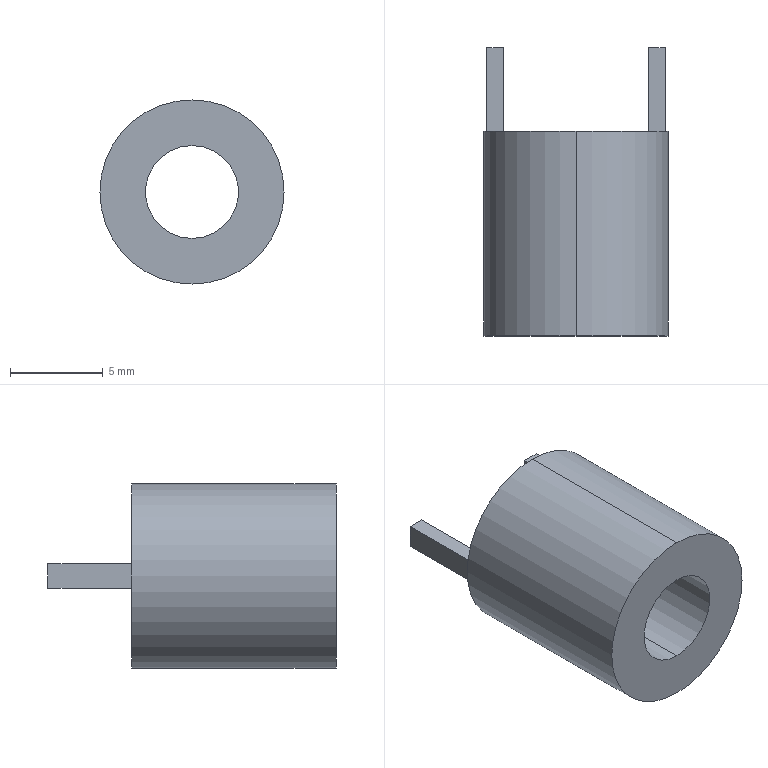Part | STEP file | 1 solid | 16 faces | box 9.9 x 15.5 x 9.9 mm | volume 641.291 mm3 | plane 12 | cylinder 4 | commonest cylinder face diameters 5 x2 9.9 x2
STEP:
#1=CARTESIAN_POINT('',(0.,0.,0.));
#2=DIRECTION('',(0.,0.,1.));
#3=DIRECTION('',(1.,0.,0.));
#4=AXIS2_PLACEMENT_3D('',#1,#2,#3);
#5=CARTESIAN_POINT('',(0.,0.,2.5));
#6=VERTEX_POINT('',#5);
#7=CARTESIAN_POINT('',(0.,11.,2.5));
#8=VERTEX_POINT('',#7);
#9=CARTESIAN_POINT('',(0.,11.,2.5));
#10=DIRECTION('',(0.,1.,0.));
#11=VECTOR('',#10,1.);
#12=LINE('',#9,#11);
#13=CARTESIAN_POINT('',(0.,11.,0.));
#14=DIRECTION('',(0.,1.,0.));
#15=DIRECTION('',(0.,0.,1.));
#16=AXIS2_PLACEMENT_3D('',#13,#14,#15);
#17=CYLINDRICAL_SURFACE('',#16,2.5);
#18=CARTESIAN_POINT('',(6.283,0.));
#19=DIRECTION('',(0.,1.));
#20=VECTOR('',#19,1.);
#21=LINE('',#18,#20);
#22=(GEOMETRIC_REPRESENTATION_CONTEXT(2)PARAMETRIC_REPRESENTATION_CONTEXT()REPRESENTATION_CONTEXT('',''));
#23=DEFINITIONAL_REPRESENTATION('',(#21),#22);
#24=PCURVE('',#17,#23);
#25=CARTESIAN_POINT('',(0.,11.,0.));
#26=DIRECTION('',(0.,1.,0.));
#27=DIRECTION('',(0.,0.,1.));
#28=AXIS2_PLACEMENT_3D('',#25,#26,#27);
#29=CYLINDRICAL_SURFACE('',#28,2.5);
#30=CARTESIAN_POINT('',(0.,0.));
#31=DIRECTION('',(0.,1.));
#32=VECTOR('',#31,1.);
#33=LINE('',#30,#32);
#34=(GEOMETRIC_REPRESENTATION_CONTEXT(2)PARAMETRIC_REPRESENTATION_CONTEXT()REPRESENTATION_CONTEXT('',''));
#35=DEFINITIONAL_REPRESENTATION('',(#33),#34);
#36=PCURVE('',#29,#35);
#37=SURFACE_CURVE('',#12,(#24,#36),.PCURVE_S1.);
#38=EDGE_CURVE('',#6,#8,#37,.T.);
#39=ORIENTED_EDGE('',*,*,#38,.T.);
#40=CARTESIAN_POINT('',(0.,11.,-2.5));
#41=VERTEX_POINT('',#40);
#42=CARTESIAN_POINT('',(0.,11.,0.));
#43=DIRECTION('',(0.,1.,0.));
#44=DIRECTION('',(0.,0.,1.));
#45=AXIS2_PLACEMENT_3D('',#42,#43,#44);
#46=CIRCLE('',#45,2.5);
#47=CARTESIAN_POINT('',(0.,0.));
#48=DIRECTION('',(1.,0.));
#49=VECTOR('',#48,1.);
#50=LINE('',#47,#49);
#51=(GEOMETRIC_REPRESENTATION_CONTEXT(2)PARAMETRIC_REPRESENTATION_CONTEXT()REPRESENTATION_CONTEXT('',''));
#52=DEFINITIONAL_REPRESENTATION('',(#50),#51);
#53=PCURVE('',#17,#52);
#54=CARTESIAN_POINT('',(0.,11.,0.));
#55=DIRECTION('',(0.,1.,0.));
#56=DIRECTION('',(0.,0.,1.));
#57=AXIS2_PLACEMENT_3D('',#54,#55,#56);
#58=PLANE('',#57);
#59=CARTESIAN_POINT('',(0.,0.));
#60=DIRECTION('',(1.,0.));
#61=AXIS2_PLACEMENT_2D('',#59,#60);
#62=CIRCLE('',#61,2.5);
#63=(GEOMETRIC_REPRESENTATION_CONTEXT(2)PARAMETRIC_REPRESENTATION_CONTEXT()REPRESENTATION_CONTEXT('',''));
#64=DEFINITIONAL_REPRESENTATION('',(#62),#63);
#65=PCURVE('',#58,#64);
#66=SURFACE_CURVE('',#46,(#53,#65),.PCURVE_S1.);
#67=EDGE_CURVE('',#41,#8,#66,.T.);
#68=ORIENTED_EDGE('',*,*,#67,.F.);
#69=CARTESIAN_POINT('',(0.,0.,-2.5));
#70=VERTEX_POINT('',#69);
#71=CARTESIAN_POINT('',(0.,11.,-2.5));
#72=DIRECTION('',(0.,1.,0.));
#73=VECTOR('',#72,1.);
#74=LINE('',#71,#73);
#75=CARTESIAN_POINT('',(3.142,0.));
#76=DIRECTION('',(0.,1.));
#77=VECTOR('',#76,1.);
#78=LINE('',#75,#77);
#79=(GEOMETRIC_REPRESENTATION_CONTEXT(2)PARAMETRIC_REPRESENTATION_CONTEXT()REPRESENTATION_CONTEXT('',''));
#80=DEFINITIONAL_REPRESENTATION('',(#78),#79);
#81=PCURVE('',#17,#80);
#82=CARTESIAN_POINT('',(3.142,0.));
#83=DIRECTION('',(0.,1.));
#84=VECTOR('',#83,1.);
#85=LINE('',#82,#84);
#86=(GEOMETRIC_REPRESENTATION_CONTEXT(2)PARAMETRIC_REPRESENTATION_CONTEXT()REPRESENTATION_CONTEXT('',''));
#87=DEFINITIONAL_REPRESENTATION('',(#85),#86);
#88=PCURVE('',#29,#87);
#89=SURFACE_CURVE('',#74,(#81,#88),.PCURVE_S1.);
#90=EDGE_CURVE('',#70,#41,#89,.T.);
#91=ORIENTED_EDGE('',*,*,#90,.F.);
#92=CARTESIAN_POINT('',(0.,0.,0.));
#93=DIRECTION('',(0.,1.,0.));
#94=DIRECTION('',(0.,0.,1.));
#95=AXIS2_PLACEMENT_3D('',#92,#93,#94);
#96=CIRCLE('',#95,2.5);
#97=CARTESIAN_POINT('',(0.,-11.));
#98=DIRECTION('',(1.,0.));
#99=VECTOR('',#98,1.);
#100=LINE('',#97,#99);
#101=(GEOMETRIC_REPRESENTATION_CONTEXT(2)PARAMETRIC_REPRESENTATION_CONTEXT()REPRESENTATION_CONTEXT('',''));
#102=DEFINITIONAL_REPRESENTATION('',(#100),#101);
#103=PCURVE('',#17,#102);
#104=CARTESIAN_POINT('',(0.,0.,0.));
#105=DIRECTION('',(0.,1.,0.));
#106=DIRECTION('',(0.,0.,1.));
#107=AXIS2_PLACEMENT_3D('',#104,#105,#106);
#108=PLANE('',#107);
#109=CARTESIAN_POINT('',(0.,0.));
#110=DIRECTION('',(1.,0.));
#111=AXIS2_PLACEMENT_2D('',#109,#110);
#112=CIRCLE('',#111,2.5);
#113=(GEOMETRIC_REPRESENTATION_CONTEXT(2)PARAMETRIC_REPRESENTATION_CONTEXT()REPRESENTATION_CONTEXT('',''));
#114=DEFINITIONAL_REPRESENTATION('',(#112),#113);
#115=PCURVE('',#108,#114);
#116=SURFACE_CURVE('',#96,(#103,#115),.PCURVE_S1.);
#117=EDGE_CURVE('',#70,#6,#116,.T.);
#118=ORIENTED_EDGE('',*,*,#117,.T.);
#119=EDGE_LOOP('',(#39,#68,#91,#118));
#120=FACE_BOUND('',#119,.F.);
#121=ADVANCED_FACE('',(#120),#17,.F.);
#122=CARTESIAN_POINT('',(0.,11.,4.95));
#123=VERTEX_POINT('',#122);
#124=CARTESIAN_POINT('',(0.,11.,-4.95));
#125=VERTEX_POINT('',#124);
#126=CARTESIAN_POINT('',(0.,11.,0.));
#127=DIRECTION('',(0.,1.,0.));
#128=DIRECTION('',(0.,0.,1.));
#129=AXIS2_PLACEMENT_3D('',#126,#127,#128);
#130=CIRCLE('',#129,4.95);
#131=CARTESIAN_POINT('',(0.,11.,0.));
#132=DIRECTION('',(0.,-1.,0.));
#133=DIRECTION('',(0.,0.,-1.));
#134=AXIS2_PLACEMENT_3D('',#131,#132,#133);
#135=CYLINDRICAL_SURFACE('',#134,4.95);
#136=CARTESIAN_POINT('',(3.142,0.));
#137=DIRECTION('',(-1.,0.));
#138=VECTOR('',#137,1.);
#139=LINE('',#136,#138);
#140=(GEOMETRIC_REPRESENTATION_CONTEXT(2)PARAMETRIC_REPRESENTATION_CONTEXT()REPRESENTATION_CONTEXT('',''));
#141=DEFINITIONAL_REPRESENTATION('',(#139),#140);
#142=PCURVE('',#135,#141);
#143=CARTESIAN_POINT('',(0.,0.));
#144=DIRECTION('',(1.,0.));
#145=AXIS2_PLACEMENT_2D('',#143,#144);
#146=CIRCLE('',#145,4.95);
#147=(GEOMETRIC_REPRESENTATION_CONTEXT(2)PARAMETRIC_REPRESENTATION_CONTEXT()REPRESENTATION_CONTEXT('',''));
#148=DEFINITIONAL_REPRESENTATION('',(#146),#147);
#149=PCURVE('',#58,#148);
#150=SURFACE_CURVE('',#130,(#142,#149),.PCURVE_S1.);
#151=EDGE_CURVE('',#123,#125,#150,.T.);
#152=ORIENTED_EDGE('',*,*,#151,.F.);
#153=CARTESIAN_POINT('',(0.,0.,4.95));
#154=VERTEX_POINT('',#153);
#155=CARTESIAN_POINT('',(0.,11.,4.95));
#156=DIRECTION('',(0.,-1.,0.));
#157=VECTOR('',#156,1.);
#158=LINE('',#155,#157);
#159=CARTESIAN_POINT('',(3.142,0.));
#160=DIRECTION('',(0.,1.));
#161=VECTOR('',#160,1.);
#162=LINE('',#159,#161);
#163=(GEOMETRIC_REPRESENTATION_CONTEXT(2)PARAMETRIC_REPRESENTATION_CONTEXT()REPRESENTATION_CONTEXT('',''));
#164=DEFINITIONAL_REPRESENTATION('',(#162),#163);
#165=PCURVE('',#135,#164);
#166=CARTESIAN_POINT('',(0.,11.,0.));
#167=DIRECTION('',(0.,-1.,0.));
#168=DIRECTION('',(0.,0.,-1.));
#169=AXIS2_PLACEMENT_3D('',#166,#167,#168);
#170=CYLINDRICAL_SURFACE('',#169,4.95);
#171=CARTESIAN_POINT('',(3.142,0.));
#172=DIRECTION('',(0.,1.));
#173=VECTOR('',#172,1.);
#174=LINE('',#171,#173);
#175=(GEOMETRIC_REPRESENTATION_CONTEXT(2)PARAMETRIC_REPRESENTATION_CONTEXT()REPRESENTATION_CONTEXT('',''));
#176=DEFINITIONAL_REPRESENTATION('',(#174),#175);
#177=PCURVE('',#170,#176);
#178=SURFACE_CURVE('',#158,(#165,#177),.PCURVE_S1.);
#179=EDGE_CURVE('',#123,#154,#178,.T.);
#180=ORIENTED_EDGE('',*,*,#179,.T.);
#181=CARTESIAN_POINT('',(0.,0.,-4.95));
#182=VERTEX_POINT('',#181);
#183=CARTESIAN_POINT('',(0.,0.,0.));
#184=DIRECTION('',(0.,1.,0.));
#185=DIRECTION('',(0.,0.,1.));
#186=AXIS2_PLACEMENT_3D('',#183,#184,#185);
#187=CIRCLE('',#186,4.95);
#188=CARTESIAN_POINT('',(3.142,11.));
#189=DIRECTION('',(-1.,0.));
#190=VECTOR('',#189,1.);
#191=LINE('',#188,#190);
#192=(GEOMETRIC_REPRESENTATION_CONTEXT(2)PARAMETRIC_REPRESENTATION_CONTEXT()REPRESENTATION_CONTEXT('',''));
#193=DEFINITIONAL_REPRESENTATION('',(#191),#192);
#194=PCURVE('',#135,#193);
#195=CARTESIAN_POINT('',(0.,0.));
#196=DIRECTION('',(1.,0.));
#197=AXIS2_PLACEMENT_2D('',#195,#196);
#198=CIRCLE('',#197,4.95);
#199=(GEOMETRIC_REPRESENTATION_CONTEXT(2)PARAMETRIC_REPRESENTATION_CONTEXT()REPRESENTATION_CONTEXT('',''));
#200=DEFINITIONAL_REPRESENTATION('',(#198),#199);
#201=PCURVE('',#108,#200);
#202=SURFACE_CURVE('',#187,(#194,#201),.PCURVE_S1.);
#203=EDGE_CURVE('',#154,#182,#202,.T.);
#204=ORIENTED_EDGE('',*,*,#203,.T.);
#205=CARTESIAN_POINT('',(0.,11.,-4.95));
#206=DIRECTION('',(0.,-1.,0.));
#207=VECTOR('',#206,1.);
#208=LINE('',#205,#207);
#209=CARTESIAN_POINT('',(0.,0.));
#210=DIRECTION('',(0.,1.));
#211=VECTOR('',#210,1.);
#212=LINE('',#209,#211);
#213=(GEOMETRIC_REPRESENTATION_CONTEXT(2)PARAMETRIC_REPRESENTATION_CONTEXT()REPRESENTATION_CONTEXT('',''));
#214=DEFINITIONAL_REPRESENTATION('',(#212),#213);
#215=PCURVE('',#135,#214);
#216=CARTESIAN_POINT('',(6.283,0.));
#217=DIRECTION('',(0.,1.));
#218=VECTOR('',#217,1.);
#219=LINE('',#216,#218);
#220=(GEOMETRIC_REPRESENTATION_CONTEXT(2)PARAMETRIC_REPRESENTATION_CONTEXT()REPRESENTATION_CONTEXT('',''));
#221=DEFINITIONAL_REPRESENTATION('',(#219),#220);
#222=PCURVE('',#170,#221);
#223=SURFACE_CURVE('',#208,(#215,#222),.PCURVE_S1.);
#224=EDGE_CURVE('',#125,#182,#223,.T.);
#225=ORIENTED_EDGE('',*,*,#224,.F.);
#226=EDGE_LOOP('',(#152,#180,#204,#225));
#227=FACE_BOUND('',#226,.T.);
#228=ADVANCED_FACE('',(#227),#135,.T.);
#229=ORIENTED_EDGE('',*,*,#179,.F.);
#230=CARTESIAN_POINT('',(0.,11.,0.));
#231=DIRECTION('',(0.,1.,0.));
#232=DIRECTION('',(0.,0.,1.));
#233=AXIS2_PLACEMENT_3D('',#230,#231,#232);
#234=CIRCLE('',#233,4.95);
#235=CARTESIAN_POINT('',(9.425,0.));
#236=DIRECTION('',(-1.,0.));
#237=VECTOR('',#236,1.);
#238=LINE('',#235,#237);
#239=(GEOMETRIC_REPRESENTATION_CONTEXT(2)PARAMETRIC_REPRESENTATION_CONTEXT()REPRESENTATION_CONTEXT('',''));
#240=DEFINITIONAL_REPRESENTATION('',(#238),#239);
#241=PCURVE('',#170,#240);
#242=CARTESIAN_POINT('',(0.,0.));
#243=DIRECTION('',(1.,0.));
#244=AXIS2_PLACEMENT_2D('',#242,#243);
#245=CIRCLE('',#244,4.95);
#246=(GEOMETRIC_REPRESENTATION_CONTEXT(2)PARAMETRIC_REPRESENTATION_CONTEXT()REPRESENTATION_CONTEXT('',''));
#247=DEFINITIONAL_REPRESENTATION('',(#245),#246);
#248=PCURVE('',#58,#247);
#249=SURFACE_CURVE('',#234,(#241,#248),.PCURVE_S1.);
#250=EDGE_CURVE('',#125,#123,#249,.T.);
#251=ORIENTED_EDGE('',*,*,#250,.F.);
#252=ORIENTED_EDGE('',*,*,#224,.T.);
#253=CARTESIAN_POINT('',(0.,0.,0.));
#254=DIRECTION('',(0.,1.,0.));
#255=DIRECTION('',(0.,0.,1.));
#256=AXIS2_PLACEMENT_3D('',#253,#254,#255);
#257=CIRCLE('',#256,4.95);
#258=CARTESIAN_POINT('',(9.425,11.));
#259=DIRECTION('',(-1.,0.));
#260=VECTOR('',#259,1.);
#261=LINE('',#258,#260);
#262=(GEOMETRIC_REPRESENTATION_CONTEXT(2)PARAMETRIC_REPRESENTATION_CONTEXT()REPRESENTATION_CONTEXT('',''));
#263=DEFINITIONAL_REPRESENTATION('',(#261),#262);
#264=PCURVE('',#170,#263);
#265=CARTESIAN_POINT('',(0.,0.));
#266=DIRECTION('',(1.,0.));
#267=AXIS2_PLACEMENT_2D('',#265,#266);
#268=CIRCLE('',#267,4.95);
#269=(GEOMETRIC_REPRESENTATION_CONTEXT(2)PARAMETRIC_REPRESENTATION_CONTEXT()REPRESENTATION_CONTEXT('',''));
#270=DEFINITIONAL_REPRESENTATION('',(#268),#269);
#271=PCURVE('',#108,#270);
#272=SURFACE_CURVE('',#257,(#264,#271),.PCURVE_S1.);
#273=EDGE_CURVE('',#182,#154,#272,.T.);
#274=ORIENTED_EDGE('',*,*,#273,.T.);
#275=EDGE_LOOP('',(#229,#251,#252,#274));
#276=FACE_BOUND('',#275,.T.);
#277=ADVANCED_FACE('',(#276),#170,.T.);
#278=CARTESIAN_POINT('',(4.8,11.,-0.65));
#279=VERTEX_POINT('',#278);
#280=CARTESIAN_POINT('',(3.9,11.,-0.65));
#281=VERTEX_POINT('',#280);
#282=CARTESIAN_POINT('',(4.907,11.,-0.65));
#283=DIRECTION('',(-1.,0.,0.));
#284=VECTOR('',#283,1.);
#285=LINE('',#282,#284);
#286=CARTESIAN_POINT('',(-0.65,4.907));
#287=DIRECTION('',(0.,-1.));
#288=VECTOR('',#287,1.);
#289=LINE('',#286,#288);
#290=(GEOMETRIC_REPRESENTATION_CONTEXT(2)PARAMETRIC_REPRESENTATION_CONTEXT()REPRESENTATION_CONTEXT('',''));
#291=DEFINITIONAL_REPRESENTATION('',(#289),#290);
#292=PCURVE('',#58,#291);
#293=CARTESIAN_POINT('',(4.907,15.5,-0.65));
#294=DIRECTION('',(0.,0.,1.));
#295=DIRECTION('',(1.,0.,0.));
#296=AXIS2_PLACEMENT_3D('',#293,#294,#295);
#297=PLANE('',#296);
#298=CARTESIAN_POINT('',(0.,-4.5));
#299=DIRECTION('',(-1.,0.));
#300=VECTOR('',#299,1.);
#301=LINE('',#298,#300);
#302=(GEOMETRIC_REPRESENTATION_CONTEXT(2)PARAMETRIC_REPRESENTATION_CONTEXT()REPRESENTATION_CONTEXT('',''));
#303=DEFINITIONAL_REPRESENTATION('',(#301),#302);
#304=PCURVE('',#297,#303);
#305=SURFACE_CURVE('',#285,(#292,#304),.PCURVE_S1.);
#306=EDGE_CURVE('',#279,#281,#305,.T.);
#307=ORIENTED_EDGE('',*,*,#306,.F.);
#308=CARTESIAN_POINT('',(4.8,11.,0.65));
#309=VERTEX_POINT('',#308);
#310=CARTESIAN_POINT('',(4.8,11.,-0.65));
#311=DIRECTION('',(0.,0.,-1.));
#312=VECTOR('',#311,1.);
#313=LINE('',#310,#312);
#314=CARTESIAN_POINT('',(-0.65,4.8));
#315=DIRECTION('',(-1.,0.));
#316=VECTOR('',#315,1.);
#317=LINE('',#314,#316);
#318=(GEOMETRIC_REPRESENTATION_CONTEXT(2)PARAMETRIC_REPRESENTATION_CONTEXT()REPRESENTATION_CONTEXT('',''));
#319=DEFINITIONAL_REPRESENTATION('',(#317),#318);
#320=PCURVE('',#58,#319);
#321=CARTESIAN_POINT('',(4.8,9.691,-0.65));
#322=DIRECTION('',(-1.,0.,0.));
#323=DIRECTION('',(0.,0.,1.));
#324=AXIS2_PLACEMENT_3D('',#321,#322,#323);
#325=PLANE('',#324);
#326=CARTESIAN_POINT('',(0.,1.309));
#327=DIRECTION('',(-1.,0.));
#328=VECTOR('',#327,1.);
#329=LINE('',#326,#328);
#330=(GEOMETRIC_REPRESENTATION_CONTEXT(2)PARAMETRIC_REPRESENTATION_CONTEXT()REPRESENTATION_CONTEXT('',''));
#331=DEFINITIONAL_REPRESENTATION('',(#329),#330);
#332=PCURVE('',#325,#331);
#333=SURFACE_CURVE('',#313,(#320,#332),.PCURVE_S1.);
#334=EDGE_CURVE('',#309,#279,#333,.T.);
#335=ORIENTED_EDGE('',*,*,#334,.F.);
#336=CARTESIAN_POINT('',(3.9,11.,0.65));
#337=VERTEX_POINT('',#336);
#338=CARTESIAN_POINT('',(3.9,11.,0.65));
#339=DIRECTION('',(1.,0.,0.));
#340=VECTOR('',#339,1.);
#341=LINE('',#338,#340);
#342=CARTESIAN_POINT('',(0.65,3.9));
#343=DIRECTION('',(0.,1.));
#344=VECTOR('',#343,1.);
#345=LINE('',#342,#344);
#346=(GEOMETRIC_REPRESENTATION_CONTEXT(2)PARAMETRIC_REPRESENTATION_CONTEXT()REPRESENTATION_CONTEXT('',''));
#347=DEFINITIONAL_REPRESENTATION('',(#345),#346);
#348=PCURVE('',#58,#347);
#349=CARTESIAN_POINT('',(3.9,15.5,0.65));
#350=DIRECTION('',(0.,0.,-1.));
#351=DIRECTION('',(-1.,0.,0.));
#352=AXIS2_PLACEMENT_3D('',#349,#350,#351);
#353=PLANE('',#352);
#354=CARTESIAN_POINT('',(0.,-4.5));
#355=DIRECTION('',(-1.,0.));
#356=VECTOR('',#355,1.);
#357=LINE('',#354,#356);
#358=(GEOMETRIC_REPRESENTATION_CONTEXT(2)PARAMETRIC_REPRESENTATION_CONTEXT()REPRESENTATION_CONTEXT('',''));
#359=DEFINITIONAL_REPRESENTATION('',(#357),#358);
#360=PCURVE('',#353,#359);
#361=SURFACE_CURVE('',#341,(#348,#360),.PCURVE_S1.);
#362=EDGE_CURVE('',#337,#309,#361,.T.);
#363=ORIENTED_EDGE('',*,*,#362,.F.);
#364=CARTESIAN_POINT('',(3.9,11.,-0.65));
#365=DIRECTION('',(0.,0.,1.));
#366=VECTOR('',#365,1.);
#367=LINE('',#364,#366);
#368=CARTESIAN_POINT('',(-0.65,3.9));
#369=DIRECTION('',(1.,0.));
#370=VECTOR('',#369,1.);
#371=LINE('',#368,#370);
#372=(GEOMETRIC_REPRESENTATION_CONTEXT(2)PARAMETRIC_REPRESENTATION_CONTEXT()REPRESENTATION_CONTEXT('',''));
#373=DEFINITIONAL_REPRESENTATION('',(#371),#372);
#374=PCURVE('',#58,#373);
#375=CARTESIAN_POINT('',(3.9,15.5,-0.65));
#376=DIRECTION('',(1.,0.,0.));
#377=DIRECTION('',(0.,0.,-1.));
#378=AXIS2_PLACEMENT_3D('',#375,#376,#377);
#379=PLANE('',#378);
#380=CARTESIAN_POINT('',(0.,-4.5));
#381=DIRECTION('',(-1.,0.));
#382=VECTOR('',#381,1.);
#383=LINE('',#380,#382);
#384=(GEOMETRIC_REPRESENTATION_CONTEXT(2)PARAMETRIC_REPRESENTATION_CONTEXT()REPRESENTATION_CONTEXT('',''));
#385=DEFINITIONAL_REPRESENTATION('',(#383),#384);
#386=PCURVE('',#379,#385);
#387=SURFACE_CURVE('',#367,(#374,#386),.PCURVE_S1.);
#388=EDGE_CURVE('',#281,#337,#387,.T.);
#389=ORIENTED_EDGE('',*,*,#388,.F.);
#390=EDGE_LOOP('',(#307,#335,#363,#389));
#391=FACE_BOUND('',#390,.T.);
#392=CARTESIAN_POINT('',(-4.8,11.,-0.65));
#393=VERTEX_POINT('',#392);
#394=CARTESIAN_POINT('',(-4.8,11.,0.65));
#395=VERTEX_POINT('',#394);
#396=CARTESIAN_POINT('',(-4.8,11.,-0.65));
#397=DIRECTION('',(0.,0.,1.));
#398=VECTOR('',#397,1.);
#399=LINE('',#396,#398);
#400=CARTESIAN_POINT('',(-0.65,-4.8));
#401=DIRECTION('',(1.,0.));
#402=VECTOR('',#401,1.);
#403=LINE('',#400,#402);
#404=(GEOMETRIC_REPRESENTATION_CONTEXT(2)PARAMETRIC_REPRESENTATION_CONTEXT()REPRESENTATION_CONTEXT('',''));
#405=DEFINITIONAL_REPRESENTATION('',(#403),#404);
#406=PCURVE('',#58,#405);
#407=CARTESIAN_POINT('',(-4.8,9.691,-0.65));
#408=DIRECTION('',(1.,0.,0.));
#409=DIRECTION('',(0.,0.,-1.));
#410=AXIS2_PLACEMENT_3D('',#407,#408,#409);
#411=PLANE('',#410);
#412=CARTESIAN_POINT('',(0.,1.309));
#413=DIRECTION('',(-1.,0.));
#414=VECTOR('',#413,1.);
#415=LINE('',#412,#414);
#416=(GEOMETRIC_REPRESENTATION_CONTEXT(2)PARAMETRIC_REPRESENTATION_CONTEXT()REPRESENTATION_CONTEXT('',''));
#417=DEFINITIONAL_REPRESENTATION('',(#415),#416);
#418=PCURVE('',#411,#417);
#419=SURFACE_CURVE('',#399,(#406,#418),.PCURVE_S1.);
#420=EDGE_CURVE('',#393,#395,#419,.T.);
#421=ORIENTED_EDGE('',*,*,#420,.F.);
#422=CARTESIAN_POINT('',(-3.9,11.,-0.65));
#423=VERTEX_POINT('',#422);
#424=CARTESIAN_POINT('',(-4.907,11.,-0.65));
#425=DIRECTION('',(-1.,0.,0.));
#426=VECTOR('',#425,1.);
#427=LINE('',#424,#426);
#428=CARTESIAN_POINT('',(-0.65,-4.907));
#429=DIRECTION('',(0.,-1.));
#430=VECTOR('',#429,1.);
#431=LINE('',#428,#430);
#432=(GEOMETRIC_REPRESENTATION_CONTEXT(2)PARAMETRIC_REPRESENTATION_CONTEXT()REPRESENTATION_CONTEXT('',''));
#433=DEFINITIONAL_REPRESENTATION('',(#431),#432);
#434=PCURVE('',#58,#433);
#435=CARTESIAN_POINT('',(-4.907,15.5,-0.65));
#436=DIRECTION('',(0.,0.,1.));
#437=DIRECTION('',(1.,0.,0.));
#438=AXIS2_PLACEMENT_3D('',#435,#436,#437);
#439=PLANE('',#438);
#440=CARTESIAN_POINT('',(0.,-4.5));
#441=DIRECTION('',(-1.,0.));
#442=VECTOR('',#441,1.);
#443=LINE('',#440,#442);
#444=(GEOMETRIC_REPRESENTATION_CONTEXT(2)PARAMETRIC_REPRESENTATION_CONTEXT()REPRESENTATION_CONTEXT('',''));
#445=DEFINITIONAL_REPRESENTATION('',(#443),#444);
#446=PCURVE('',#439,#445);
#447=SURFACE_CURVE('',#427,(#434,#446),.PCURVE_S1.);
#448=EDGE_CURVE('',#423,#393,#447,.T.);
#449=ORIENTED_EDGE('',*,*,#448,.F.);
#450=CARTESIAN_POINT('',(-3.9,11.,0.65));
#451=VERTEX_POINT('',#450);
#452=CARTESIAN_POINT('',(-3.9,11.,-0.65));
#453=DIRECTION('',(0.,0.,-1.));
#454=VECTOR('',#453,1.);
#455=LINE('',#452,#454);
#456=CARTESIAN_POINT('',(-0.65,-3.9));
#457=DIRECTION('',(-1.,0.));
#458=VECTOR('',#457,1.);
#459=LINE('',#456,#458);
#460=(GEOMETRIC_REPRESENTATION_CONTEXT(2)PARAMETRIC_REPRESENTATION_CONTEXT()REPRESENTATION_CONTEXT('',''));
#461=DEFINITIONAL_REPRESENTATION('',(#459),#460);
#462=PCURVE('',#58,#461);
#463=CARTESIAN_POINT('',(-3.9,15.5,-0.65));
#464=DIRECTION('',(-1.,0.,0.));
#465=DIRECTION('',(0.,0.,1.));
#466=AXIS2_PLACEMENT_3D('',#463,#464,#465);
#467=PLANE('',#466);
#468=CARTESIAN_POINT('',(0.,-4.5));
#469=DIRECTION('',(-1.,0.));
#470=VECTOR('',#469,1.);
#471=LINE('',#468,#470);
#472=(GEOMETRIC_REPRESENTATION_CONTEXT(2)PARAMETRIC_REPRESENTATION_CONTEXT()REPRESENTATION_CONTEXT('',''));
#473=DEFINITIONAL_REPRESENTATION('',(#471),#472);
#474=PCURVE('',#467,#473);
#475=SURFACE_CURVE('',#455,(#462,#474),.PCURVE_S1.);
#476=EDGE_CURVE('',#451,#423,#475,.T.);
#477=ORIENTED_EDGE('',*,*,#476,.F.);
#478=CARTESIAN_POINT('',(-3.9,11.,0.65));
#479=DIRECTION('',(1.,0.,0.));
#480=VECTOR('',#479,1.);
#481=LINE('',#478,#480);
#482=CARTESIAN_POINT('',(0.65,-3.9));
#483=DIRECTION('',(0.,1.));
#484=VECTOR('',#483,1.);
#485=LINE('',#482,#484);
#486=(GEOMETRIC_REPRESENTATION_CONTEXT(2)PARAMETRIC_REPRESENTATION_CONTEXT()REPRESENTATION_CONTEXT('',''));
#487=DEFINITIONAL_REPRESENTATION('',(#485),#486);
#488=PCURVE('',#58,#487);
#489=CARTESIAN_POINT('',(-3.9,15.5,0.65));
#490=DIRECTION('',(0.,0.,-1.));
#491=DIRECTION('',(-1.,0.,0.));
#492=AXIS2_PLACEMENT_3D('',#489,#490,#491);
#493=PLANE('',#492);
#494=CARTESIAN_POINT('',(0.,-4.5));
#495=DIRECTION('',(-1.,0.));
#496=VECTOR('',#495,1.);
#497=LINE('',#494,#496);
#498=(GEOMETRIC_REPRESENTATION_CONTEXT(2)PARAMETRIC_REPRESENTATION_CONTEXT()REPRESENTATION_CONTEXT('',''));
#499=DEFINITIONAL_REPRESENTATION('',(#497),#498);
#500=PCURVE('',#493,#499);
#501=SURFACE_CURVE('',#481,(#488,#500),.PCURVE_S1.);
#502=EDGE_CURVE('',#395,#451,#501,.T.);
#503=ORIENTED_EDGE('',*,*,#502,.F.);
#504=EDGE_LOOP('',(#421,#449,#477,#503));
#505=FACE_BOUND('',#504,.T.);
#506=CARTESIAN_POINT('',(0.,11.,0.));
#507=DIRECTION('',(0.,1.,0.));
#508=DIRECTION('',(0.,0.,1.));
#509=AXIS2_PLACEMENT_3D('',#506,#507,#508);
#510=CIRCLE('',#509,2.5);
#511=CARTESIAN_POINT('',(0.,0.));
#512=DIRECTION('',(1.,0.));
#513=AXIS2_PLACEMENT_2D('',#511,#512);
#514=CIRCLE('',#513,2.5);
#515=(GEOMETRIC_REPRESENTATION_CONTEXT(2)PARAMETRIC_REPRESENTATION_CONTEXT()REPRESENTATION_CONTEXT('',''));
#516=DEFINITIONAL_REPRESENTATION('',(#514),#515);
#517=PCURVE('',#58,#516);
#518=CARTESIAN_POINT('',(0.,0.));
#519=DIRECTION('',(1.,0.));
#520=VECTOR('',#519,1.);
#521=LINE('',#518,#520);
#522=(GEOMETRIC_REPRESENTATION_CONTEXT(2)PARAMETRIC_REPRESENTATION_CONTEXT()REPRESENTATION_CONTEXT('',''));
#523=DEFINITIONAL_REPRESENTATION('',(#521),#522);
#524=PCURVE('',#29,#523);
#525=SURFACE_CURVE('',#510,(#517,#524),.PCURVE_S1.);
#526=EDGE_CURVE('',#8,#41,#525,.T.);
#527=ORIENTED_EDGE('',*,*,#526,.F.);
#528=ORIENTED_EDGE('',*,*,#67,.F.);
#529=EDGE_LOOP('',(#527,#528));
#530=FACE_BOUND('',#529,.T.);
#531=ORIENTED_EDGE('',*,*,#250,.T.);
#532=ORIENTED_EDGE('',*,*,#151,.T.);
#533=EDGE_LOOP('',(#531,#532));
#534=FACE_BOUND('',#533,.T.);
#535=ADVANCED_FACE('',(#391,#505,#530,#534),#58,.T.);
#536=CARTESIAN_POINT('',(0.,0.,0.));
#537=DIRECTION('',(0.,1.,0.));
#538=DIRECTION('',(0.,0.,1.));
#539=AXIS2_PLACEMENT_3D('',#536,#537,#538);
#540=CIRCLE('',#539,2.5);
#541=CARTESIAN_POINT('',(0.,0.));
#542=DIRECTION('',(1.,0.));
#543=AXIS2_PLACEMENT_2D('',#541,#542);
#544=CIRCLE('',#543,2.5);
#545=(GEOMETRIC_REPRESENTATION_CONTEXT(2)PARAMETRIC_REPRESENTATION_CONTEXT()REPRESENTATION_CONTEXT('',''));
#546=DEFINITIONAL_REPRESENTATION('',(#544),#545);
#547=PCURVE('',#108,#546);
#548=CARTESIAN_POINT('',(0.,-11.));
#549=DIRECTION('',(1.,0.));
#550=VECTOR('',#549,1.);
#551=LINE('',#548,#550);
#552=(GEOMETRIC_REPRESENTATION_CONTEXT(2)PARAMETRIC_REPRESENTATION_CONTEXT()REPRESENTATION_CONTEXT('',''));
#553=DEFINITIONAL_REPRESENTATION('',(#551),#552);
#554=PCURVE('',#29,#553);
#555=SURFACE_CURVE('',#540,(#547,#554),.PCURVE_S1.);
#556=EDGE_CURVE('',#6,#70,#555,.T.);
#557=ORIENTED_EDGE('',*,*,#556,.T.);
#558=ORIENTED_EDGE('',*,*,#117,.T.);
#559=EDGE_LOOP('',(#557,#558));
#560=FACE_BOUND('',#559,.T.);
#561=ORIENTED_EDGE('',*,*,#273,.F.);
#562=ORIENTED_EDGE('',*,*,#203,.F.);
#563=EDGE_LOOP('',(#561,#562));
#564=FACE_BOUND('',#563,.T.);
#565=ADVANCED_FACE('',(#560,#564),#108,.F.);
#566=ORIENTED_EDGE('',*,*,#526,.F.);
#567=ORIENTED_EDGE('',*,*,#38,.F.);
#568=ORIENTED_EDGE('',*,*,#556,.T.);
#569=ORIENTED_EDGE('',*,*,#90,.T.);
#570=EDGE_LOOP('',(#566,#567,#568,#569));
#571=FACE_BOUND('',#570,.F.);
#572=ADVANCED_FACE('',(#571),#29,.F.);
#573=CARTESIAN_POINT('',(4.8,15.5,-0.65));
#574=VERTEX_POINT('',#573);
#575=CARTESIAN_POINT('',(3.9,15.5,-0.65));
#576=VERTEX_POINT('',#575);
#577=CARTESIAN_POINT('',(4.907,15.5,-0.65));
#578=DIRECTION('',(-1.,0.,0.));
#579=VECTOR('',#578,1.);
#580=LINE('',#577,#579);
#581=CARTESIAN_POINT('',(0.,0.));
#582=DIRECTION('',(-1.,0.));
#583=VECTOR('',#582,1.);
#584=LINE('',#581,#583);
#585=(GEOMETRIC_REPRESENTATION_CONTEXT(2)PARAMETRIC_REPRESENTATION_CONTEXT()REPRESENTATION_CONTEXT('',''));
#586=DEFINITIONAL_REPRESENTATION('',(#584),#585);
#587=PCURVE('',#297,#586);
#588=CARTESIAN_POINT('',(0.,15.5,0.));
#589=DIRECTION('',(0.,1.,0.));
#590=DIRECTION('',(0.,0.,1.));
#591=AXIS2_PLACEMENT_3D('',#588,#589,#590);
#592=PLANE('',#591);
#593=CARTESIAN_POINT('',(-0.65,4.907));
#594=DIRECTION('',(0.,-1.));
#595=VECTOR('',#594,1.);
#596=LINE('',#593,#595);
#597=(GEOMETRIC_REPRESENTATION_CONTEXT(2)PARAMETRIC_REPRESENTATION_CONTEXT()REPRESENTATION_CONTEXT('',''));
#598=DEFINITIONAL_REPRESENTATION('',(#596),#597);
#599=PCURVE('',#592,#598);
#600=SURFACE_CURVE('',#580,(#587,#599),.PCURVE_S1.);
#601=EDGE_CURVE('',#574,#576,#600,.T.);
#602=ORIENTED_EDGE('',*,*,#601,.F.);
#603=CARTESIAN_POINT('',(4.8,9.691,-0.65));
#604=DIRECTION('',(0.,1.,0.));
#605=VECTOR('',#604,1.);
#606=LINE('',#603,#605);
#607=CARTESIAN_POINT('',(-0.1071,-5.809));
#608=DIRECTION('',(0.,1.));
#609=VECTOR('',#608,1.);
#610=LINE('',#607,#609);
#611=(GEOMETRIC_REPRESENTATION_CONTEXT(2)PARAMETRIC_REPRESENTATION_CONTEXT()REPRESENTATION_CONTEXT('',''));
#612=DEFINITIONAL_REPRESENTATION('',(#610),#611);
#613=PCURVE('',#297,#612);
#614=CARTESIAN_POINT('',(0.,0.));
#615=DIRECTION('',(0.,1.));
#616=VECTOR('',#615,1.);
#617=LINE('',#614,#616);
#618=(GEOMETRIC_REPRESENTATION_CONTEXT(2)PARAMETRIC_REPRESENTATION_CONTEXT()REPRESENTATION_CONTEXT('',''));
#619=DEFINITIONAL_REPRESENTATION('',(#617),#618);
#620=PCURVE('',#325,#619);
#621=SURFACE_CURVE('',#606,(#613,#620),.PCURVE_S1.);
#622=EDGE_CURVE('',#279,#574,#621,.T.);
#623=ORIENTED_EDGE('',*,*,#622,.F.);
#624=ORIENTED_EDGE('',*,*,#306,.T.);
#625=CARTESIAN_POINT('',(3.9,15.5,-0.65));
#626=DIRECTION('',(0.,-1.,0.));
#627=VECTOR('',#626,1.);
#628=LINE('',#625,#627);
#629=CARTESIAN_POINT('',(-1.007,0.));
#630=DIRECTION('',(0.,-1.));
#631=VECTOR('',#630,1.);
#632=LINE('',#629,#631);
#633=(GEOMETRIC_REPRESENTATION_CONTEXT(2)PARAMETRIC_REPRESENTATION_CONTEXT()REPRESENTATION_CONTEXT('',''));
#634=DEFINITIONAL_REPRESENTATION('',(#632),#633);
#635=PCURVE('',#297,#634);
#636=CARTESIAN_POINT('',(0.,0.));
#637=DIRECTION('',(0.,-1.));
#638=VECTOR('',#637,1.);
#639=LINE('',#636,#638);
#640=(GEOMETRIC_REPRESENTATION_CONTEXT(2)PARAMETRIC_REPRESENTATION_CONTEXT()REPRESENTATION_CONTEXT('',''));
#641=DEFINITIONAL_REPRESENTATION('',(#639),#640);
#642=PCURVE('',#379,#641);
#643=SURFACE_CURVE('',#628,(#635,#642),.PCURVE_S1.);
#644=EDGE_CURVE('',#576,#281,#643,.T.);
#645=ORIENTED_EDGE('',*,*,#644,.F.);
#646=EDGE_LOOP('',(#602,#623,#624,#645));
#647=FACE_BOUND('',#646,.T.);
#648=ADVANCED_FACE('',(#647),#297,.F.);
#649=ORIENTED_EDGE('',*,*,#388,.T.);
#650=CARTESIAN_POINT('',(3.9,15.5,0.65));
#651=VERTEX_POINT('',#650);
#652=CARTESIAN_POINT('',(3.9,15.5,0.65));
#653=DIRECTION('',(0.,-1.,0.));
#654=VECTOR('',#653,1.);
#655=LINE('',#652,#654);
#656=CARTESIAN_POINT('',(-1.3,0.));
#657=DIRECTION('',(0.,-1.));
#658=VECTOR('',#657,1.);
#659=LINE('',#656,#658);
#660=(GEOMETRIC_REPRESENTATION_CONTEXT(2)PARAMETRIC_REPRESENTATION_CONTEXT()REPRESENTATION_CONTEXT('',''));
#661=DEFINITIONAL_REPRESENTATION('',(#659),#660);
#662=PCURVE('',#379,#661);
#663=CARTESIAN_POINT('',(0.,0.));
#664=DIRECTION('',(0.,-1.));
#665=VECTOR('',#664,1.);
#666=LINE('',#663,#665);
#667=(GEOMETRIC_REPRESENTATION_CONTEXT(2)PARAMETRIC_REPRESENTATION_CONTEXT()REPRESENTATION_CONTEXT('',''));
#668=DEFINITIONAL_REPRESENTATION('',(#666),#667);
#669=PCURVE('',#353,#668);
#670=SURFACE_CURVE('',#655,(#662,#669),.PCURVE_S1.);
#671=EDGE_CURVE('',#651,#337,#670,.T.);
#672=ORIENTED_EDGE('',*,*,#671,.F.);
#673=CARTESIAN_POINT('',(3.9,15.5,-0.65));
#674=DIRECTION('',(0.,0.,1.));
#675=VECTOR('',#674,1.);
#676=LINE('',#673,#675);
#677=CARTESIAN_POINT('',(0.,0.));
#678=DIRECTION('',(-1.,0.));
#679=VECTOR('',#678,1.);
#680=LINE('',#677,#679);
#681=(GEOMETRIC_REPRESENTATION_CONTEXT(2)PARAMETRIC_REPRESENTATION_CONTEXT()REPRESENTATION_CONTEXT('',''));
#682=DEFINITIONAL_REPRESENTATION('',(#680),#681);
#683=PCURVE('',#379,#682);
#684=CARTESIAN_POINT('',(-0.65,3.9));
#685=DIRECTION('',(1.,0.));
#686=VECTOR('',#685,1.);
#687=LINE('',#684,#686);
#688=(GEOMETRIC_REPRESENTATION_CONTEXT(2)PARAMETRIC_REPRESENTATION_CONTEXT()REPRESENTATION_CONTEXT('',''));
#689=DEFINITIONAL_REPRESENTATION('',(#687),#688);
#690=PCURVE('',#592,#689);
#691=SURFACE_CURVE('',#676,(#683,#690),.PCURVE_S1.);
#692=EDGE_CURVE('',#576,#651,#691,.T.);
#693=ORIENTED_EDGE('',*,*,#692,.F.);
#694=ORIENTED_EDGE('',*,*,#644,.T.);
#695=EDGE_LOOP('',(#649,#672,#693,#694));
#696=FACE_BOUND('',#695,.T.);
#697=ADVANCED_FACE('',(#696),#379,.F.);
#698=ORIENTED_EDGE('',*,*,#362,.T.);
#699=CARTESIAN_POINT('',(4.8,15.5,0.65));
#700=VERTEX_POINT('',#699);
#701=CARTESIAN_POINT('',(4.8,9.691,0.65));
#702=DIRECTION('',(0.,1.,0.));
#703=VECTOR('',#702,1.);
#704=LINE('',#701,#703);
#705=CARTESIAN_POINT('',(-0.9,-5.809));
#706=DIRECTION('',(0.,1.));
#707=VECTOR('',#706,1.);
#708=LINE('',#705,#707);
#709=(GEOMETRIC_REPRESENTATION_CONTEXT(2)PARAMETRIC_REPRESENTATION_CONTEXT()REPRESENTATION_CONTEXT('',''));
#710=DEFINITIONAL_REPRESENTATION('',(#708),#709);
#711=PCURVE('',#353,#710);
#712=CARTESIAN_POINT('',(1.3,0.));
#713=DIRECTION('',(0.,1.));
#714=VECTOR('',#713,1.);
#715=LINE('',#712,#714);
#716=(GEOMETRIC_REPRESENTATION_CONTEXT(2)PARAMETRIC_REPRESENTATION_CONTEXT()REPRESENTATION_CONTEXT('',''));
#717=DEFINITIONAL_REPRESENTATION('',(#715),#716);
#718=PCURVE('',#325,#717);
#719=SURFACE_CURVE('',#704,(#711,#718),.PCURVE_S1.);
#720=EDGE_CURVE('',#309,#700,#719,.T.);
#721=ORIENTED_EDGE('',*,*,#720,.T.);
#722=CARTESIAN_POINT('',(3.9,15.5,0.65));
#723=DIRECTION('',(1.,0.,0.));
#724=VECTOR('',#723,1.);
#725=LINE('',#722,#724);
#726=CARTESIAN_POINT('',(0.,0.));
#727=DIRECTION('',(-1.,0.));
#728=VECTOR('',#727,1.);
#729=LINE('',#726,#728);
#730=(GEOMETRIC_REPRESENTATION_CONTEXT(2)PARAMETRIC_REPRESENTATION_CONTEXT()REPRESENTATION_CONTEXT('',''));
#731=DEFINITIONAL_REPRESENTATION('',(#729),#730);
#732=PCURVE('',#353,#731);
#733=CARTESIAN_POINT('',(0.65,3.9));
#734=DIRECTION('',(0.,1.));
#735=VECTOR('',#734,1.);
#736=LINE('',#733,#735);
#737=(GEOMETRIC_REPRESENTATION_CONTEXT(2)PARAMETRIC_REPRESENTATION_CONTEXT()REPRESENTATION_CONTEXT('',''));
#738=DEFINITIONAL_REPRESENTATION('',(#736),#737);
#739=PCURVE('',#592,#738);
#740=SURFACE_CURVE('',#725,(#732,#739),.PCURVE_S1.);
#741=EDGE_CURVE('',#651,#700,#740,.T.);
#742=ORIENTED_EDGE('',*,*,#741,.F.);
#743=ORIENTED_EDGE('',*,*,#671,.T.);
#744=EDGE_LOOP('',(#698,#721,#742,#743));
#745=FACE_BOUND('',#744,.T.);
#746=ADVANCED_FACE('',(#745),#353,.F.);
#747=CARTESIAN_POINT('',(4.8,15.5,-0.65));
#748=DIRECTION('',(0.,0.,1.));
#749=VECTOR('',#748,1.);
#750=LINE('',#747,#749);
#751=CARTESIAN_POINT('',(-0.65,4.8));
#752=DIRECTION('',(1.,0.));
#753=VECTOR('',#752,1.);
#754=LINE('',#751,#753);
#755=(GEOMETRIC_REPRESENTATION_CONTEXT(2)PARAMETRIC_REPRESENTATION_CONTEXT()REPRESENTATION_CONTEXT('',''));
#756=DEFINITIONAL_REPRESENTATION('',(#754),#755);
#757=PCURVE('',#592,#756);
#758=CARTESIAN_POINT('',(0.,5.809));
#759=DIRECTION('',(1.,0.));
#760=VECTOR('',#759,1.);
#761=LINE('',#758,#760);
#762=(GEOMETRIC_REPRESENTATION_CONTEXT(2)PARAMETRIC_REPRESENTATION_CONTEXT()REPRESENTATION_CONTEXT('',''));
#763=DEFINITIONAL_REPRESENTATION('',(#761),#762);
#764=PCURVE('',#325,#763);
#765=SURFACE_CURVE('',#750,(#757,#764),.PCURVE_S1.);
#766=EDGE_CURVE('',#574,#700,#765,.T.);
#767=ORIENTED_EDGE('',*,*,#766,.F.);
#768=ORIENTED_EDGE('',*,*,#601,.T.);
#769=ORIENTED_EDGE('',*,*,#692,.T.);
#770=ORIENTED_EDGE('',*,*,#741,.T.);
#771=EDGE_LOOP('',(#767,#768,#769,#770));
#772=FACE_BOUND('',#771,.T.);
#773=ADVANCED_FACE('',(#772),#592,.T.);
#774=ORIENTED_EDGE('',*,*,#476,.T.);
#775=CARTESIAN_POINT('',(-3.9,15.5,-0.65));
#776=VERTEX_POINT('',#775);
#777=CARTESIAN_POINT('',(-3.9,15.5,-0.65));
#778=DIRECTION('',(0.,-1.,0.));
#779=VECTOR('',#778,1.);
#780=LINE('',#777,#779);
#781=CARTESIAN_POINT('',(0.,0.));
#782=DIRECTION('',(0.,-1.));
#783=VECTOR('',#782,1.);
#784=LINE('',#781,#783);
#785=(GEOMETRIC_REPRESENTATION_CONTEXT(2)PARAMETRIC_REPRESENTATION_CONTEXT()REPRESENTATION_CONTEXT('',''));
#786=DEFINITIONAL_REPRESENTATION('',(#784),#785);
#787=PCURVE('',#467,#786);
#788=CARTESIAN_POINT('',(1.007,0.));
#789=DIRECTION('',(0.,-1.));
#790=VECTOR('',#789,1.);
#791=LINE('',#788,#790);
#792=(GEOMETRIC_REPRESENTATION_CONTEXT(2)PARAMETRIC_REPRESENTATION_CONTEXT()REPRESENTATION_CONTEXT('',''));
#793=DEFINITIONAL_REPRESENTATION('',(#791),#792);
#794=PCURVE('',#439,#793);
#795=SURFACE_CURVE('',#780,(#787,#794),.PCURVE_S1.);
#796=EDGE_CURVE('',#776,#423,#795,.T.);
#797=ORIENTED_EDGE('',*,*,#796,.F.);
#798=CARTESIAN_POINT('',(-3.9,15.5,0.65));
#799=VERTEX_POINT('',#798);
#800=CARTESIAN_POINT('',(-3.9,15.5,-0.65));
#801=DIRECTION('',(0.,0.,-1.));
#802=VECTOR('',#801,1.);
#803=LINE('',#800,#802);
#804=CARTESIAN_POINT('',(0.,0.));
#805=DIRECTION('',(-1.,0.));
#806=VECTOR('',#805,1.);
#807=LINE('',#804,#806);
#808=(GEOMETRIC_REPRESENTATION_CONTEXT(2)PARAMETRIC_REPRESENTATION_CONTEXT()REPRESENTATION_CONTEXT('',''));
#809=DEFINITIONAL_REPRESENTATION('',(#807),#808);
#810=PCURVE('',#467,#809);
#811=CARTESIAN_POINT('',(0.,15.5,0.));
#812=DIRECTION('',(0.,1.,0.));
#813=DIRECTION('',(0.,0.,1.));
#814=AXIS2_PLACEMENT_3D('',#811,#812,#813);
#815=PLANE('',#814);
#816=CARTESIAN_POINT('',(-0.65,-3.9));
#817=DIRECTION('',(-1.,0.));
#818=VECTOR('',#817,1.);
#819=LINE('',#816,#818);
#820=(GEOMETRIC_REPRESENTATION_CONTEXT(2)PARAMETRIC_REPRESENTATION_CONTEXT()REPRESENTATION_CONTEXT('',''));
#821=DEFINITIONAL_REPRESENTATION('',(#819),#820);
#822=PCURVE('',#815,#821);
#823=SURFACE_CURVE('',#803,(#810,#822),.PCURVE_S1.);
#824=EDGE_CURVE('',#799,#776,#823,.T.);
#825=ORIENTED_EDGE('',*,*,#824,.F.);
#826=CARTESIAN_POINT('',(-3.9,15.5,0.65));
#827=DIRECTION('',(0.,-1.,0.));
#828=VECTOR('',#827,1.);
#829=LINE('',#826,#828);
#830=CARTESIAN_POINT('',(1.3,0.));
#831=DIRECTION('',(0.,-1.));
#832=VECTOR('',#831,1.);
#833=LINE('',#830,#832);
#834=(GEOMETRIC_REPRESENTATION_CONTEXT(2)PARAMETRIC_REPRESENTATION_CONTEXT()REPRESENTATION_CONTEXT('',''));
#835=DEFINITIONAL_REPRESENTATION('',(#833),#834);
#836=PCURVE('',#467,#835);
#837=CARTESIAN_POINT('',(0.,0.));
#838=DIRECTION('',(0.,-1.));
#839=VECTOR('',#838,1.);
#840=LINE('',#837,#839);
#841=(GEOMETRIC_REPRESENTATION_CONTEXT(2)PARAMETRIC_REPRESENTATION_CONTEXT()REPRESENTATION_CONTEXT('',''));
#842=DEFINITIONAL_REPRESENTATION('',(#840),#841);
#843=PCURVE('',#493,#842);
#844=SURFACE_CURVE('',#829,(#836,#843),.PCURVE_S1.);
#845=EDGE_CURVE('',#799,#451,#844,.T.);
#846=ORIENTED_EDGE('',*,*,#845,.T.);
#847=EDGE_LOOP('',(#774,#797,#825,#846));
#848=FACE_BOUND('',#847,.T.);
#849=ADVANCED_FACE('',(#848),#467,.F.);
#850=ORIENTED_EDGE('',*,*,#448,.T.);
#851=CARTESIAN_POINT('',(-4.8,15.5,-0.65));
#852=VERTEX_POINT('',#851);
#853=CARTESIAN_POINT('',(-4.8,9.691,-0.65));
#854=DIRECTION('',(0.,1.,0.));
#855=VECTOR('',#854,1.);
#856=LINE('',#853,#855);
#857=CARTESIAN_POINT('',(0.1071,-5.809));
#858=DIRECTION('',(0.,1.));
#859=VECTOR('',#858,1.);
#860=LINE('',#857,#859);
#861=(GEOMETRIC_REPRESENTATION_CONTEXT(2)PARAMETRIC_REPRESENTATION_CONTEXT()REPRESENTATION_CONTEXT('',''));
#862=DEFINITIONAL_REPRESENTATION('',(#860),#861);
#863=PCURVE('',#439,#862);
#864=CARTESIAN_POINT('',(0.,0.));
#865=DIRECTION('',(0.,1.));
#866=VECTOR('',#865,1.);
#867=LINE('',#864,#866);
#868=(GEOMETRIC_REPRESENTATION_CONTEXT(2)PARAMETRIC_REPRESENTATION_CONTEXT()REPRESENTATION_CONTEXT('',''));
#869=DEFINITIONAL_REPRESENTATION('',(#867),#868);
#870=PCURVE('',#411,#869);
#871=SURFACE_CURVE('',#856,(#863,#870),.PCURVE_S1.);
#872=EDGE_CURVE('',#393,#852,#871,.T.);
#873=ORIENTED_EDGE('',*,*,#872,.T.);
#874=CARTESIAN_POINT('',(-4.907,15.5,-0.65));
#875=DIRECTION('',(-1.,0.,0.));
#876=VECTOR('',#875,1.);
#877=LINE('',#874,#876);
#878=CARTESIAN_POINT('',(0.,0.));
#879=DIRECTION('',(-1.,0.));
#880=VECTOR('',#879,1.);
#881=LINE('',#878,#880);
#882=(GEOMETRIC_REPRESENTATION_CONTEXT(2)PARAMETRIC_REPRESENTATION_CONTEXT()REPRESENTATION_CONTEXT('',''));
#883=DEFINITIONAL_REPRESENTATION('',(#881),#882);
#884=PCURVE('',#439,#883);
#885=CARTESIAN_POINT('',(-0.65,-4.907));
#886=DIRECTION('',(0.,-1.));
#887=VECTOR('',#886,1.);
#888=LINE('',#885,#887);
#889=(GEOMETRIC_REPRESENTATION_CONTEXT(2)PARAMETRIC_REPRESENTATION_CONTEXT()REPRESENTATION_CONTEXT('',''));
#890=DEFINITIONAL_REPRESENTATION('',(#888),#889);
#891=PCURVE('',#815,#890);
#892=SURFACE_CURVE('',#877,(#884,#891),.PCURVE_S1.);
#893=EDGE_CURVE('',#776,#852,#892,.T.);
#894=ORIENTED_EDGE('',*,*,#893,.F.);
#895=ORIENTED_EDGE('',*,*,#796,.T.);
#896=EDGE_LOOP('',(#850,#873,#894,#895));
#897=FACE_BOUND('',#896,.T.);
#898=ADVANCED_FACE('',(#897),#439,.F.);
#899=CARTESIAN_POINT('',(-4.8,15.5,0.65));
#900=VERTEX_POINT('',#899);
#901=CARTESIAN_POINT('',(-3.9,15.5,0.65));
#902=DIRECTION('',(1.,0.,0.));
#903=VECTOR('',#902,1.);
#904=LINE('',#901,#903);
#905=CARTESIAN_POINT('',(0.,0.));
#906=DIRECTION('',(-1.,0.));
#907=VECTOR('',#906,1.);
#908=LINE('',#905,#907);
#909=(GEOMETRIC_REPRESENTATION_CONTEXT(2)PARAMETRIC_REPRESENTATION_CONTEXT()REPRESENTATION_CONTEXT('',''));
#910=DEFINITIONAL_REPRESENTATION('',(#908),#909);
#911=PCURVE('',#493,#910);
#912=CARTESIAN_POINT('',(0.65,-3.9));
#913=DIRECTION('',(0.,1.));
#914=VECTOR('',#913,1.);
#915=LINE('',#912,#914);
#916=(GEOMETRIC_REPRESENTATION_CONTEXT(2)PARAMETRIC_REPRESENTATION_CONTEXT()REPRESENTATION_CONTEXT('',''));
#917=DEFINITIONAL_REPRESENTATION('',(#915),#916);
#918=PCURVE('',#815,#917);
#919=SURFACE_CURVE('',#904,(#911,#918),.PCURVE_S1.);
#920=EDGE_CURVE('',#900,#799,#919,.T.);
#921=ORIENTED_EDGE('',*,*,#920,.F.);
#922=CARTESIAN_POINT('',(-4.8,9.691,0.65));
#923=DIRECTION('',(0.,1.,0.));
#924=VECTOR('',#923,1.);
#925=LINE('',#922,#924);
#926=CARTESIAN_POINT('',(0.9,-5.809));
#927=DIRECTION('',(0.,1.));
#928=VECTOR('',#927,1.);
#929=LINE('',#926,#928);
#930=(GEOMETRIC_REPRESENTATION_CONTEXT(2)PARAMETRIC_REPRESENTATION_CONTEXT()REPRESENTATION_CONTEXT('',''));
#931=DEFINITIONAL_REPRESENTATION('',(#929),#930);
#932=PCURVE('',#493,#931);
#933=CARTESIAN_POINT('',(-1.3,0.));
#934=DIRECTION('',(0.,1.));
#935=VECTOR('',#934,1.);
#936=LINE('',#933,#935);
#937=(GEOMETRIC_REPRESENTATION_CONTEXT(2)PARAMETRIC_REPRESENTATION_CONTEXT()REPRESENTATION_CONTEXT('',''));
#938=DEFINITIONAL_REPRESENTATION('',(#936),#937);
#939=PCURVE('',#411,#938);
#940=SURFACE_CURVE('',#925,(#932,#939),.PCURVE_S1.);
#941=EDGE_CURVE('',#395,#900,#940,.T.);
#942=ORIENTED_EDGE('',*,*,#941,.F.);
#943=ORIENTED_EDGE('',*,*,#502,.T.);
#944=ORIENTED_EDGE('',*,*,#845,.F.);
#945=EDGE_LOOP('',(#921,#942,#943,#944));
#946=FACE_BOUND('',#945,.T.);
#947=ADVANCED_FACE('',(#946),#493,.F.);
#948=CARTESIAN_POINT('',(-4.8,15.5,-0.65));
#949=DIRECTION('',(0.,0.,-1.));
#950=VECTOR('',#949,1.);
#951=LINE('',#948,#950);
#952=CARTESIAN_POINT('',(-0.65,-4.8));
#953=DIRECTION('',(-1.,0.));
#954=VECTOR('',#953,1.);
#955=LINE('',#952,#954);
#956=(GEOMETRIC_REPRESENTATION_CONTEXT(2)PARAMETRIC_REPRESENTATION_CONTEXT()REPRESENTATION_CONTEXT('',''));
#957=DEFINITIONAL_REPRESENTATION('',(#955),#956);
#958=PCURVE('',#815,#957);
#959=CARTESIAN_POINT('',(0.,5.809));
#960=DIRECTION('',(1.,0.));
#961=VECTOR('',#960,1.);
#962=LINE('',#959,#961);
#963=(GEOMETRIC_REPRESENTATION_CONTEXT(2)PARAMETRIC_REPRESENTATION_CONTEXT()REPRESENTATION_CONTEXT('',''));
#964=DEFINITIONAL_REPRESENTATION('',(#962),#963);
#965=PCURVE('',#411,#964);
#966=SURFACE_CURVE('',#951,(#958,#965),.PCURVE_S1.);
#967=EDGE_CURVE('',#900,#852,#966,.T.);
#968=ORIENTED_EDGE('',*,*,#967,.F.);
#969=ORIENTED_EDGE('',*,*,#920,.T.);
#970=ORIENTED_EDGE('',*,*,#824,.T.);
#971=ORIENTED_EDGE('',*,*,#893,.T.);
#972=EDGE_LOOP('',(#968,#969,#970,#971));
#973=FACE_BOUND('',#972,.T.);
#974=ADVANCED_FACE('',(#973),#815,.T.);
#975=ORIENTED_EDGE('',*,*,#420,.T.);
#976=ORIENTED_EDGE('',*,*,#941,.T.);
#977=ORIENTED_EDGE('',*,*,#967,.T.);
#978=ORIENTED_EDGE('',*,*,#872,.F.);
#979=EDGE_LOOP('',(#975,#976,#977,#978));
#980=FACE_BOUND('',#979,.T.);
#981=ADVANCED_FACE('',(#980),#411,.F.);
#982=ORIENTED_EDGE('',*,*,#334,.T.);
#983=ORIENTED_EDGE('',*,*,#622,.T.);
#984=ORIENTED_EDGE('',*,*,#766,.T.);
#985=ORIENTED_EDGE('',*,*,#720,.F.);
#986=EDGE_LOOP('',(#982,#983,#984,#985));
#987=FACE_BOUND('',#986,.T.);
#988=ADVANCED_FACE('',(#987),#325,.F.);
#989=CLOSED_SHELL('',(#121,#228,#277,#535,#565,#572,#648,#697,#746,#773,#849,#898,#947,#974,#981,#988));
#990=MANIFOLD_SOLID_BREP('',#989);
#991=(LENGTH_UNIT()NAMED_UNIT(*)SI_UNIT(.MILLI.,.METRE.));
#992=UNCERTAINTY_MEASURE_WITH_UNIT(LENGTH_MEASURE(0.0000001),#991,'','');
#993=(NAMED_UNIT(*)PLANE_ANGLE_UNIT()SI_UNIT($,.RADIAN.));
#994=(NAMED_UNIT(*)SI_UNIT($,.STERADIAN.)SOLID_ANGLE_UNIT());
#995=(GEOMETRIC_REPRESENTATION_CONTEXT(3)GLOBAL_UNCERTAINTY_ASSIGNED_CONTEXT((#992))GLOBAL_UNIT_ASSIGNED_CONTEXT((#991,#993,#994))REPRESENTATION_CONTEXT('',''));
#996=ADVANCED_BREP_SHAPE_REPRESENTATION('',(#4,#990),#995);